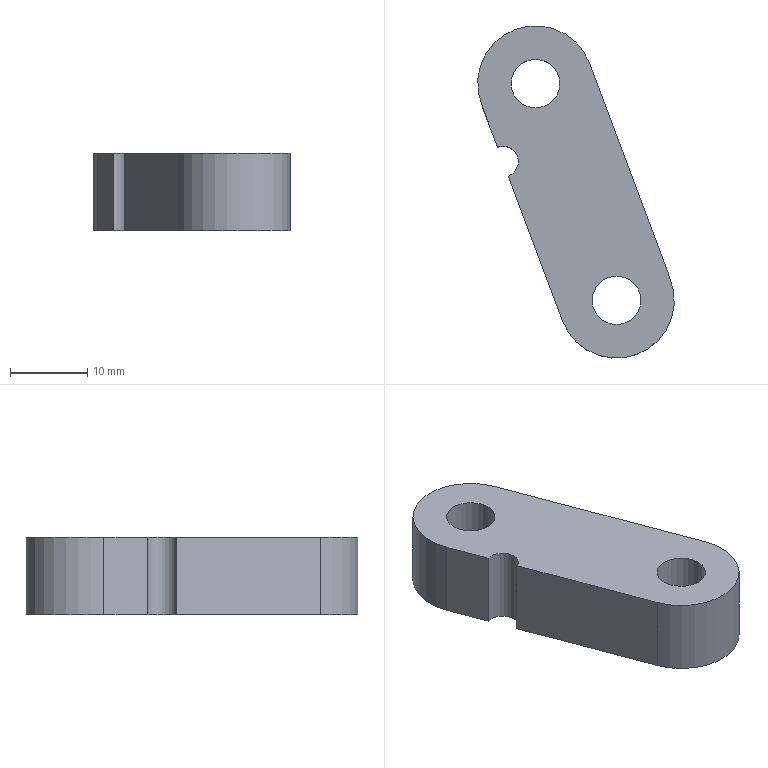Part | NX | features solid 2 | 1 solid | 10 faces | box 25.506 x 43.1 x 10 mm | volume 5581 mm3 | plane 5 | cylinder 5 | commonest cylinder face diameters 6.3 x2 15 x2 4.001 x1
STEP:
#1=CARTESIAN_POINT('',(342.943,-34.747,15.002));
#2=VERTEX_POINT('',#1);
#3=CARTESIAN_POINT('',(345.044,-40.367,15.002));
#4=VERTEX_POINT('',#3);
#5=CARTESIAN_POINT('',(344.256,-38.26,15.002));
#6=DIRECTION('',(0.3502,-0.9367,-0.000000001));
#7=VECTOR('',#6,1000.);
#8=LINE('',#5,#7);
#9=EDGE_CURVE('',#2,#4,#8,.T.);
#10=ORIENTED_EDGE('',*,*,#9,.T.);
#11=CARTESIAN_POINT('',(345.044,-40.367,25.002));
#12=VERTEX_POINT('',#11);
#13=CARTESIAN_POINT('',(345.044,-40.367,25.002));
#14=DIRECTION('',(-0.000000103,-0.000000037,-1.));
#15=VECTOR('',#14,1000.);
#16=LINE('',#13,#15);
#17=EDGE_CURVE('',#12,#4,#16,.T.);
#18=ORIENTED_EDGE('',*,*,#17,.F.);
#19=CARTESIAN_POINT('',(342.943,-34.747,25.002));
#20=VERTEX_POINT('',#19);
#21=CARTESIAN_POINT('',(344.256,-38.26,25.002));
#22=DIRECTION('',(0.3502,-0.9367,-0.000000001));
#23=VECTOR('',#22,1000.);
#24=LINE('',#21,#23);
#25=EDGE_CURVE('',#20,#12,#24,.T.);
#26=ORIENTED_EDGE('',*,*,#25,.F.);
#27=CARTESIAN_POINT('',(342.943,-34.747,25.002));
#28=DIRECTION('',(-0.000000103,-0.000000037,-1.));
#29=VECTOR('',#28,1000.);
#30=LINE('',#27,#29);
#31=EDGE_CURVE('',#20,#2,#30,.T.);
#32=ORIENTED_EDGE('',*,*,#31,.T.);
#33=EDGE_LOOP('',(#10,#18,#26,#32));
#34=FACE_BOUND('',#33,.T.);
#35=CARTESIAN_POINT('',(344.256,-38.26,25.002));
#36=DIRECTION('',(0.9367,0.3502,-0.000000109));
#37=DIRECTION('',(0.3502,-0.9367,0.));
#38=AXIS2_PLACEMENT_3D('',#35,#36,#37);
#39=PLANE('',#38);
#40=ADVANCED_FACE('',(#34),#39,.F.);
#41=CARTESIAN_POINT('',(346.445,-44.114,15.002));
#42=VERTEX_POINT('',#41);
#43=CARTESIAN_POINT('',(345.744,-42.241,15.002));
#44=DIRECTION('',(-0.000000103,-0.000000037,-1.));
#45=DIRECTION('',(1.,0.,-0.000000103));
#46=AXIS2_PLACEMENT_3D('',#43,#44,#45);
#47=CIRCLE('',#46,2.001);
#48=EDGE_CURVE('',#4,#42,#47,.T.);
#49=ORIENTED_EDGE('',*,*,#48,.T.);
#50=CARTESIAN_POINT('',(346.445,-44.114,25.002));
#51=VERTEX_POINT('',#50);
#52=CARTESIAN_POINT('',(346.445,-44.114,25.002));
#53=DIRECTION('',(-0.000000103,-0.000000037,-1.));
#54=VECTOR('',#53,1000.);
#55=LINE('',#52,#54);
#56=EDGE_CURVE('',#51,#42,#55,.T.);
#57=ORIENTED_EDGE('',*,*,#56,.F.);
#58=CARTESIAN_POINT('',(345.744,-42.241,25.002));
#59=DIRECTION('',(-0.000000103,-0.000000037,-1.));
#60=DIRECTION('',(1.,0.,-0.000000103));
#61=AXIS2_PLACEMENT_3D('',#58,#59,#60);
#62=CIRCLE('',#61,2.001);
#63=EDGE_CURVE('',#12,#51,#62,.T.);
#64=ORIENTED_EDGE('',*,*,#63,.F.);
#65=ORIENTED_EDGE('',*,*,#17,.T.);
#66=EDGE_LOOP('',(#49,#57,#64,#65));
#67=FACE_BOUND('',#66,.T.);
#68=CARTESIAN_POINT('',(345.744,-42.241,25.002));
#69=DIRECTION('',(-0.000000103,-0.000000037,-1.));
#70=DIRECTION('',(1.,0.,-0.000000103));
#71=AXIS2_PLACEMENT_3D('',#68,#69,#70);
#72=CYLINDRICAL_SURFACE('',#71,2.001);
#73=ADVANCED_FACE('',(#67),#72,.F.);
#74=CARTESIAN_POINT('',(353.449,-62.847,15.002));
#75=VERTEX_POINT('',#74);
#76=CARTESIAN_POINT('',(344.256,-38.26,15.002));
#77=DIRECTION('',(0.3502,-0.9367,-0.000000001));
#78=VECTOR('',#77,1000.);
#79=LINE('',#76,#78);
#80=EDGE_CURVE('',#42,#75,#79,.T.);
#81=ORIENTED_EDGE('',*,*,#80,.T.);
#82=CARTESIAN_POINT('',(353.449,-62.847,25.002));
#83=VERTEX_POINT('',#82);
#84=CARTESIAN_POINT('',(353.449,-62.847,25.002));
#85=DIRECTION('',(-0.000000103,-0.000000037,-1.));
#86=VECTOR('',#85,1000.);
#87=LINE('',#84,#86);
#88=EDGE_CURVE('',#83,#75,#87,.T.);
#89=ORIENTED_EDGE('',*,*,#88,.F.);
#90=CARTESIAN_POINT('',(344.256,-38.26,25.002));
#91=DIRECTION('',(0.3502,-0.9367,-0.000000001));
#92=VECTOR('',#91,1000.);
#93=LINE('',#90,#92);
#94=EDGE_CURVE('',#51,#83,#93,.T.);
#95=ORIENTED_EDGE('',*,*,#94,.F.);
#96=ORIENTED_EDGE('',*,*,#56,.T.);
#97=EDGE_LOOP('',(#81,#89,#95,#96));
#98=FACE_BOUND('',#97,.T.);
#99=CARTESIAN_POINT('',(344.256,-38.26,25.002));
#100=DIRECTION('',(0.9367,0.3502,-0.000000109));
#101=DIRECTION('',(0.3502,-0.9367,0.));
#102=AXIS2_PLACEMENT_3D('',#99,#100,#101);
#103=PLANE('',#102);
#104=ADVANCED_FACE('',(#98),#103,.F.);
#105=CARTESIAN_POINT('',(367.499,-57.594,15.002));
#106=VERTEX_POINT('',#105);
#107=CARTESIAN_POINT('',(360.474,-60.221,15.002));
#108=DIRECTION('',(-0.000000103,-0.000000037,-1.));
#109=DIRECTION('',(1.,0.,-0.000000103));
#110=AXIS2_PLACEMENT_3D('',#107,#108,#109);
#111=CIRCLE('',#110,7.5);
#112=EDGE_CURVE('',#106,#75,#111,.T.);
#113=ORIENTED_EDGE('',*,*,#112,.F.);
#114=CARTESIAN_POINT('',(367.499,-57.594,25.002));
#115=VERTEX_POINT('',#114);
#116=CARTESIAN_POINT('',(367.499,-57.594,25.002));
#117=DIRECTION('',(-0.000000103,-0.000000037,-1.));
#118=VECTOR('',#117,1000.);
#119=LINE('',#116,#118);
#120=EDGE_CURVE('',#115,#106,#119,.T.);
#121=ORIENTED_EDGE('',*,*,#120,.F.);
#122=CARTESIAN_POINT('',(360.474,-60.221,25.002));
#123=DIRECTION('',(-0.000000103,-0.000000037,-1.));
#124=DIRECTION('',(1.,0.,-0.000000103));
#125=AXIS2_PLACEMENT_3D('',#122,#123,#124);
#126=CIRCLE('',#125,7.5);
#127=EDGE_CURVE('',#115,#83,#126,.T.);
#128=ORIENTED_EDGE('',*,*,#127,.T.);
#129=ORIENTED_EDGE('',*,*,#88,.T.);
#130=EDGE_LOOP('',(#113,#121,#128,#129));
#131=FACE_BOUND('',#130,.T.);
#132=CARTESIAN_POINT('',(360.474,-60.221,25.002));
#133=DIRECTION('',(-0.000000103,-0.000000037,-1.));
#134=DIRECTION('',(1.,0.,-0.000000103));
#135=AXIS2_PLACEMENT_3D('',#132,#133,#134);
#136=CYLINDRICAL_SURFACE('',#135,7.5);
#137=ADVANCED_FACE('',(#131),#136,.T.);
#138=CARTESIAN_POINT('',(356.993,-29.494,15.002));
#139=VERTEX_POINT('',#138);
#140=CARTESIAN_POINT('',(358.306,-33.007,15.002));
#141=DIRECTION('',(0.3502,-0.9367,-0.000000001));
#142=VECTOR('',#141,1000.);
#143=LINE('',#140,#142);
#144=EDGE_CURVE('',#139,#106,#143,.T.);
#145=ORIENTED_EDGE('',*,*,#144,.F.);
#146=CARTESIAN_POINT('',(356.993,-29.494,25.002));
#147=VERTEX_POINT('',#146);
#148=CARTESIAN_POINT('',(356.993,-29.494,25.002));
#149=DIRECTION('',(-0.000000103,-0.000000037,-1.));
#150=VECTOR('',#149,1000.);
#151=LINE('',#148,#150);
#152=EDGE_CURVE('',#147,#139,#151,.T.);
#153=ORIENTED_EDGE('',*,*,#152,.F.);
#154=CARTESIAN_POINT('',(358.306,-33.007,25.002));
#155=DIRECTION('',(0.3502,-0.9367,-0.000000001));
#156=VECTOR('',#155,1000.);
#157=LINE('',#154,#156);
#158=EDGE_CURVE('',#147,#115,#157,.T.);
#159=ORIENTED_EDGE('',*,*,#158,.T.);
#160=ORIENTED_EDGE('',*,*,#120,.T.);
#161=EDGE_LOOP('',(#145,#153,#159,#160));
#162=FACE_BOUND('',#161,.T.);
#163=CARTESIAN_POINT('',(358.306,-33.007,25.002));
#164=DIRECTION('',(0.9367,0.3502,-0.000000109));
#165=DIRECTION('',(0.3502,-0.9367,0.));
#166=AXIS2_PLACEMENT_3D('',#163,#164,#165);
#167=PLANE('',#166);
#168=ADVANCED_FACE('',(#162),#167,.T.);
#169=CARTESIAN_POINT('',(363.624,-60.221,25.002));
#170=VERTEX_POINT('',#169);
#171=CARTESIAN_POINT('',(360.474,-60.221,25.002));
#172=DIRECTION('',(-0.000000103,-0.000000037,-1.));
#173=DIRECTION('',(1.,0.,-0.000000103));
#174=AXIS2_PLACEMENT_3D('',#171,#172,#173);
#175=CIRCLE('',#174,3.15);
#176=EDGE_CURVE('',#170,#170,#175,.T.);
#177=ORIENTED_EDGE('',*,*,#176,.F.);
#178=EDGE_LOOP('',(#177));
#179=FACE_BOUND('',#178,.T.);
#180=CARTESIAN_POINT('',(363.624,-60.221,15.002));
#181=VERTEX_POINT('',#180);
#182=CARTESIAN_POINT('',(360.474,-60.221,15.002));
#183=DIRECTION('',(-0.000000103,-0.000000037,-1.));
#184=DIRECTION('',(1.,0.,-0.000000103));
#185=AXIS2_PLACEMENT_3D('',#182,#183,#184);
#186=CIRCLE('',#185,3.15);
#187=EDGE_CURVE('',#181,#181,#186,.T.);
#188=ORIENTED_EDGE('',*,*,#187,.T.);
#189=EDGE_LOOP('',(#188));
#190=FACE_BOUND('',#189,.T.);
#191=CARTESIAN_POINT('',(360.474,-60.221,25.002));
#192=DIRECTION('',(-0.000000103,-0.000000037,-1.));
#193=DIRECTION('',(1.,0.,-0.000000103));
#194=AXIS2_PLACEMENT_3D('',#191,#192,#193);
#195=CYLINDRICAL_SURFACE('',#194,3.15);
#196=ADVANCED_FACE('',(#179,#190),#195,.F.);
#197=CARTESIAN_POINT('',(353.118,-32.121,25.002));
#198=VERTEX_POINT('',#197);
#199=CARTESIAN_POINT('',(349.968,-32.121,25.002));
#200=DIRECTION('',(0.000000103,0.000000037,1.));
#201=DIRECTION('',(1.,0.,-0.000000103));
#202=AXIS2_PLACEMENT_3D('',#199,#200,#201);
#203=CIRCLE('',#202,3.15);
#204=EDGE_CURVE('',#198,#198,#203,.T.);
#205=ORIENTED_EDGE('',*,*,#204,.T.);
#206=EDGE_LOOP('',(#205));
#207=FACE_BOUND('',#206,.T.);
#208=CARTESIAN_POINT('',(353.118,-32.121,15.002));
#209=VERTEX_POINT('',#208);
#210=CARTESIAN_POINT('',(349.968,-32.121,15.002));
#211=DIRECTION('',(0.000000103,0.000000037,1.));
#212=DIRECTION('',(1.,0.,-0.000000103));
#213=AXIS2_PLACEMENT_3D('',#210,#211,#212);
#214=CIRCLE('',#213,3.15);
#215=EDGE_CURVE('',#209,#209,#214,.T.);
#216=ORIENTED_EDGE('',*,*,#215,.F.);
#217=EDGE_LOOP('',(#216));
#218=FACE_BOUND('',#217,.T.);
#219=CARTESIAN_POINT('',(349.968,-32.121,25.002));
#220=DIRECTION('',(-0.000000103,-0.000000037,-1.));
#221=DIRECTION('',(1.,0.,-0.000000103));
#222=AXIS2_PLACEMENT_3D('',#219,#220,#221);
#223=CYLINDRICAL_SURFACE('',#222,3.15);
#224=ADVANCED_FACE('',(#207,#218),#223,.F.);
#225=CARTESIAN_POINT('',(349.968,-32.121,15.002));
#226=DIRECTION('',(-0.000000103,-0.000000037,-1.));
#227=DIRECTION('',(-0.04361,0.999,-0.000000033));
#228=AXIS2_PLACEMENT_3D('',#225,#226,#227);
#229=CIRCLE('',#228,7.5);
#230=EDGE_CURVE('',#2,#139,#229,.T.);
#231=ORIENTED_EDGE('',*,*,#230,.F.);
#232=ORIENTED_EDGE('',*,*,#31,.F.);
#233=CARTESIAN_POINT('',(349.968,-32.121,25.002));
#234=DIRECTION('',(-0.000000103,-0.000000037,-1.));
#235=DIRECTION('',(-0.04361,0.999,-0.000000033));
#236=AXIS2_PLACEMENT_3D('',#233,#234,#235);
#237=CIRCLE('',#236,7.5);
#238=EDGE_CURVE('',#20,#147,#237,.T.);
#239=ORIENTED_EDGE('',*,*,#238,.T.);
#240=ORIENTED_EDGE('',*,*,#152,.T.);
#241=EDGE_LOOP('',(#231,#232,#239,#240));
#242=FACE_BOUND('',#241,.T.);
#243=CARTESIAN_POINT('',(349.968,-32.121,25.002));
#244=DIRECTION('',(-0.000000103,-0.000000037,-1.));
#245=DIRECTION('',(1.,0.,-0.000000103));
#246=AXIS2_PLACEMENT_3D('',#243,#244,#245);
#247=CYLINDRICAL_SURFACE('',#246,7.5);
#248=ADVANCED_FACE('',(#242),#247,.T.);
#249=ORIENTED_EDGE('',*,*,#204,.F.);
#250=EDGE_LOOP('',(#249));
#251=FACE_BOUND('',#250,.T.);
#252=ORIENTED_EDGE('',*,*,#176,.T.);
#253=EDGE_LOOP('',(#252));
#254=FACE_BOUND('',#253,.T.);
#255=ORIENTED_EDGE('',*,*,#25,.T.);
#256=ORIENTED_EDGE('',*,*,#63,.T.);
#257=ORIENTED_EDGE('',*,*,#94,.T.);
#258=ORIENTED_EDGE('',*,*,#127,.F.);
#259=ORIENTED_EDGE('',*,*,#158,.F.);
#260=ORIENTED_EDGE('',*,*,#238,.F.);
#261=EDGE_LOOP('',(#255,#256,#257,#258,#259,#260));
#262=FACE_BOUND('',#261,.T.);
#263=CARTESIAN_POINT('',(351.281,-35.633,25.002));
#264=DIRECTION('',(0.000000103,0.000000037,1.));
#265=DIRECTION('',(-0.04361,0.999,-0.000000033));
#266=AXIS2_PLACEMENT_3D('',#263,#264,#265);
#267=PLANE('',#266);
#268=ADVANCED_FACE('',(#251,#254,#262),#267,.T.);
#269=ORIENTED_EDGE('',*,*,#215,.T.);
#270=EDGE_LOOP('',(#269));
#271=FACE_BOUND('',#270,.T.);
#272=ORIENTED_EDGE('',*,*,#187,.F.);
#273=EDGE_LOOP('',(#272));
#274=FACE_BOUND('',#273,.T.);
#275=ORIENTED_EDGE('',*,*,#9,.F.);
#276=ORIENTED_EDGE('',*,*,#230,.T.);
#277=ORIENTED_EDGE('',*,*,#144,.T.);
#278=ORIENTED_EDGE('',*,*,#112,.T.);
#279=ORIENTED_EDGE('',*,*,#80,.F.);
#280=ORIENTED_EDGE('',*,*,#48,.F.);
#281=EDGE_LOOP('',(#275,#276,#277,#278,#279,#280));
#282=FACE_BOUND('',#281,.T.);
#283=CARTESIAN_POINT('',(351.281,-35.633,15.002));
#284=DIRECTION('',(0.000000103,0.000000037,1.));
#285=DIRECTION('',(-0.04361,0.999,-0.000000033));
#286=AXIS2_PLACEMENT_3D('',#283,#284,#285);
#287=PLANE('',#286);
#288=ADVANCED_FACE('',(#271,#274,#282),#287,.F.);
#289=CLOSED_SHELL('',(#40,#73,#104,#137,#168,#196,#224,#248,#268,#288));
#290=MANIFOLD_SOLID_BREP('',#289);
#291=(LENGTH_UNIT()NAMED_UNIT(*)SI_UNIT(.MILLI.,.METRE.));
#292=UNCERTAINTY_MEASURE_WITH_UNIT(LENGTH_MEASURE(0.00001),#291,'','');
#293=(NAMED_UNIT(*)PLANE_ANGLE_UNIT()SI_UNIT($,.RADIAN.));
#294=(NAMED_UNIT(*)SI_UNIT($,.STERADIAN.)SOLID_ANGLE_UNIT());
#295=(GEOMETRIC_REPRESENTATION_CONTEXT(3)GLOBAL_UNCERTAINTY_ASSIGNED_CONTEXT((#292))GLOBAL_UNIT_ASSIGNED_CONTEXT((#291,#293,#294))REPRESENTATION_CONTEXT('',''));
#296=ADVANCED_BREP_SHAPE_REPRESENTATION('',(#290),#295);